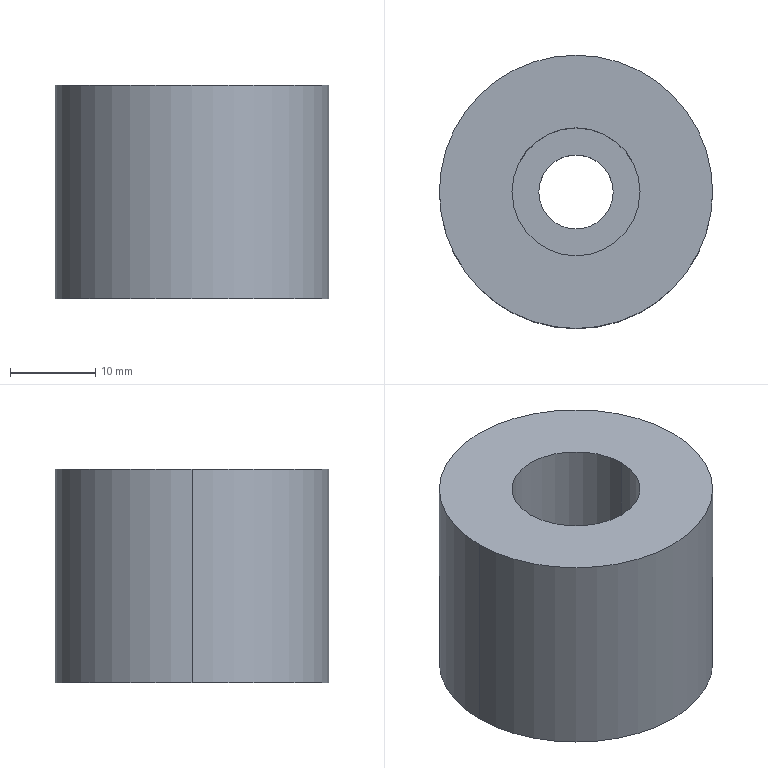Part | STEP file | 1_id1246_x_t | 1 solid | 9 faces | box 32 x 32 x 25 mm | volume 17096 mm3 | cylinder 6 | plane 3 | commonest cylinder face diameters 8.7 x2 15 x2 32 x2
STEP:
#1=CARTESIAN_POINT('',(0.,0.,0.));
#2=DIRECTION('',(0.,0.,1.));
#3=DIRECTION('',(1.,0.,0.));
#4=AXIS2_PLACEMENT_3D('',#1,#2,#3);
#5=CARTESIAN_POINT('',(181.925,338.,3.24));
#6=VERTEX_POINT('',#5);
#7=CARTESIAN_POINT('',(181.925,338.,-21.76));
#8=VERTEX_POINT('',#7);
#9=CARTESIAN_POINT('',(181.925,338.,3.24));
#10=DIRECTION('',(0.,0.,-1.));
#11=VECTOR('',#10,1.);
#12=LINE('',#9,#11);
#13=CARTESIAN_POINT('',(197.925,338.,-46.76));
#14=DIRECTION('',(0.,0.,-1.));
#15=DIRECTION('',(1.,0.,0.));
#16=AXIS2_PLACEMENT_3D('',#13,#14,#15);
#17=CYLINDRICAL_SURFACE('',#16,16.);
#18=CARTESIAN_POINT('',(3.142,-50.));
#19=DIRECTION('',(0.,1.));
#20=VECTOR('',#19,1.);
#21=LINE('',#18,#20);
#22=(GEOMETRIC_REPRESENTATION_CONTEXT(2)PARAMETRIC_REPRESENTATION_CONTEXT()REPRESENTATION_CONTEXT('',''));
#23=DEFINITIONAL_REPRESENTATION('',(#21),#22);
#24=PCURVE('',#17,#23);
#25=CARTESIAN_POINT('',(197.925,338.,-46.76));
#26=DIRECTION('',(0.,0.,-1.));
#27=DIRECTION('',(1.,0.,0.));
#28=AXIS2_PLACEMENT_3D('',#25,#26,#27);
#29=CYLINDRICAL_SURFACE('',#28,16.);
#30=CARTESIAN_POINT('',(3.142,-50.));
#31=DIRECTION('',(0.,1.));
#32=VECTOR('',#31,1.);
#33=LINE('',#30,#32);
#34=(GEOMETRIC_REPRESENTATION_CONTEXT(2)PARAMETRIC_REPRESENTATION_CONTEXT()REPRESENTATION_CONTEXT('',''));
#35=DEFINITIONAL_REPRESENTATION('',(#33),#34);
#36=PCURVE('',#29,#35);
#37=SURFACE_CURVE('',#12,(#24,#36),.PCURVE_S1.);
#38=EDGE_CURVE('',#6,#8,#37,.T.);
#39=ORIENTED_EDGE('',*,*,#38,.F.);
#40=CARTESIAN_POINT('',(213.925,338.,3.24));
#41=VERTEX_POINT('',#40);
#42=CARTESIAN_POINT('',(197.925,338.,3.24));
#43=DIRECTION('',(0.,0.,1.));
#44=DIRECTION('',(1.,0.,0.));
#45=AXIS2_PLACEMENT_3D('',#42,#43,#44);
#46=CIRCLE('',#45,16.);
#47=CARTESIAN_POINT('',(6.283,-50.));
#48=DIRECTION('',(-1.,0.));
#49=VECTOR('',#48,1.);
#50=LINE('',#47,#49);
#51=(GEOMETRIC_REPRESENTATION_CONTEXT(2)PARAMETRIC_REPRESENTATION_CONTEXT()REPRESENTATION_CONTEXT('',''));
#52=DEFINITIONAL_REPRESENTATION('',(#50),#51);
#53=PCURVE('',#17,#52);
#54=CARTESIAN_POINT('',(197.925,338.,3.24));
#55=DIRECTION('',(0.,0.,-1.));
#56=DIRECTION('',(-1.,0.,0.));
#57=AXIS2_PLACEMENT_3D('',#54,#55,#56);
#58=PLANE('',#57);
#59=CARTESIAN_POINT('',(-16.,0.));
#60=CARTESIAN_POINT('',(-16.,27.713));
#61=CARTESIAN_POINT('',(8.,13.856));
#62=CARTESIAN_POINT('',(32.,0.));
#63=CARTESIAN_POINT('',(8.,-13.856));
#64=CARTESIAN_POINT('',(-16.,-27.713));
#65=CARTESIAN_POINT('',(-16.,0.));
#66=(BOUNDED_CURVE()B_SPLINE_CURVE(2,(#59,#60,#61,#62,#63,#64,#65),.UNSPECIFIED.,.T.,.F.)B_SPLINE_CURVE_WITH_KNOTS((1,2,2,2,2,1),(-2.094,0.,2.094,4.189,6.283,8.378),.UNSPECIFIED.)CURVE()GEOMETRIC_REPRESENTATION_ITEM()RATIONAL_B_SPLINE_CURVE((1.,0.5,1.,0.5,1.,0.5,1.))REPRESENTATION_ITEM(''));
#67=(GEOMETRIC_REPRESENTATION_CONTEXT(2)PARAMETRIC_REPRESENTATION_CONTEXT()REPRESENTATION_CONTEXT('',''));
#68=DEFINITIONAL_REPRESENTATION('',(#66),#67);
#69=PCURVE('',#58,#68);
#70=SURFACE_CURVE('',#46,(#53,#69),.PCURVE_S1.);
#71=EDGE_CURVE('',#41,#6,#70,.T.);
#72=ORIENTED_EDGE('',*,*,#71,.F.);
#73=CARTESIAN_POINT('',(213.925,338.,-21.76));
#74=VERTEX_POINT('',#73);
#75=CARTESIAN_POINT('',(213.925,338.,3.24));
#76=DIRECTION('',(0.,0.,1.));
#77=VECTOR('',#76,1.);
#78=LINE('',#75,#77);
#79=CARTESIAN_POINT('',(6.283,-50.));
#80=DIRECTION('',(0.,-1.));
#81=VECTOR('',#80,1.);
#82=LINE('',#79,#81);
#83=(GEOMETRIC_REPRESENTATION_CONTEXT(2)PARAMETRIC_REPRESENTATION_CONTEXT()REPRESENTATION_CONTEXT('',''));
#84=DEFINITIONAL_REPRESENTATION('',(#82),#83);
#85=PCURVE('',#17,#84);
#86=CARTESIAN_POINT('',(0.,-50.));
#87=DIRECTION('',(0.,-1.));
#88=VECTOR('',#87,1.);
#89=LINE('',#86,#88);
#90=(GEOMETRIC_REPRESENTATION_CONTEXT(2)PARAMETRIC_REPRESENTATION_CONTEXT()REPRESENTATION_CONTEXT('',''));
#91=DEFINITIONAL_REPRESENTATION('',(#89),#90);
#92=PCURVE('',#29,#91);
#93=SURFACE_CURVE('',#78,(#85,#92),.PCURVE_S1.);
#94=EDGE_CURVE('',#74,#41,#93,.T.);
#95=ORIENTED_EDGE('',*,*,#94,.F.);
#96=CARTESIAN_POINT('',(197.925,338.,-21.76));
#97=DIRECTION('',(0.,0.,-1.));
#98=DIRECTION('',(-1.,0.,0.));
#99=AXIS2_PLACEMENT_3D('',#96,#97,#98);
#100=CIRCLE('',#99,16.);
#101=CARTESIAN_POINT('',(3.142,-25.));
#102=DIRECTION('',(1.,0.));
#103=VECTOR('',#102,1.);
#104=LINE('',#101,#103);
#105=(GEOMETRIC_REPRESENTATION_CONTEXT(2)PARAMETRIC_REPRESENTATION_CONTEXT()REPRESENTATION_CONTEXT('',''));
#106=DEFINITIONAL_REPRESENTATION('',(#104),#105);
#107=PCURVE('',#17,#106);
#108=CARTESIAN_POINT('',(197.925,338.,-21.76));
#109=DIRECTION('',(0.,0.,1.));
#110=DIRECTION('',(1.,0.,0.));
#111=AXIS2_PLACEMENT_3D('',#108,#109,#110);
#112=PLANE('',#111);
#113=CARTESIAN_POINT('',(-16.,0.));
#114=CARTESIAN_POINT('',(-16.,27.713));
#115=CARTESIAN_POINT('',(8.,13.856));
#116=CARTESIAN_POINT('',(32.,0.));
#117=CARTESIAN_POINT('',(8.,-13.856));
#118=CARTESIAN_POINT('',(-16.,-27.713));
#119=CARTESIAN_POINT('',(-16.,0.));
#120=(BOUNDED_CURVE()B_SPLINE_CURVE(2,(#113,#114,#115,#116,#117,#118,#119),.UNSPECIFIED.,.T.,.F.)B_SPLINE_CURVE_WITH_KNOTS((1,2,2,2,2,1),(-2.094,0.,2.094,4.189,6.283,8.378),.UNSPECIFIED.)CURVE()GEOMETRIC_REPRESENTATION_ITEM()RATIONAL_B_SPLINE_CURVE((1.,0.5,1.,0.5,1.,0.5,1.))REPRESENTATION_ITEM(''));
#121=(GEOMETRIC_REPRESENTATION_CONTEXT(2)PARAMETRIC_REPRESENTATION_CONTEXT()REPRESENTATION_CONTEXT('',''));
#122=DEFINITIONAL_REPRESENTATION('',(#120),#121);
#123=PCURVE('',#112,#122);
#124=SURFACE_CURVE('',#100,(#107,#123),.PCURVE_S1.);
#125=EDGE_CURVE('',#8,#74,#124,.T.);
#126=ORIENTED_EDGE('',*,*,#125,.F.);
#127=EDGE_LOOP('',(#39,#72,#95,#126));
#128=FACE_BOUND('',#127,.T.);
#129=ADVANCED_FACE('',(#128),#17,.T.);
#130=CARTESIAN_POINT('',(197.925,338.,-21.76));
#131=DIRECTION('',(0.,0.,-1.));
#132=DIRECTION('',(1.,0.,0.));
#133=AXIS2_PLACEMENT_3D('',#130,#131,#132);
#134=CIRCLE('',#133,16.);
#135=CARTESIAN_POINT('',(16.,0.));
#136=CARTESIAN_POINT('',(16.,-27.713));
#137=CARTESIAN_POINT('',(-8.,-13.856));
#138=CARTESIAN_POINT('',(-32.,0.));
#139=CARTESIAN_POINT('',(-8.,13.856));
#140=CARTESIAN_POINT('',(16.,27.713));
#141=CARTESIAN_POINT('',(16.,0.));
#142=(BOUNDED_CURVE()B_SPLINE_CURVE(2,(#135,#136,#137,#138,#139,#140,#141),.UNSPECIFIED.,.T.,.F.)B_SPLINE_CURVE_WITH_KNOTS((1,2,2,2,2,1),(-2.094,0.,2.094,4.189,6.283,8.378),.UNSPECIFIED.)CURVE()GEOMETRIC_REPRESENTATION_ITEM()RATIONAL_B_SPLINE_CURVE((1.,0.5,1.,0.5,1.,0.5,1.))REPRESENTATION_ITEM(''));
#143=(GEOMETRIC_REPRESENTATION_CONTEXT(2)PARAMETRIC_REPRESENTATION_CONTEXT()REPRESENTATION_CONTEXT('',''));
#144=DEFINITIONAL_REPRESENTATION('',(#142),#143);
#145=PCURVE('',#112,#144);
#146=CARTESIAN_POINT('',(0.,-25.));
#147=DIRECTION('',(1.,0.));
#148=VECTOR('',#147,1.);
#149=LINE('',#146,#148);
#150=(GEOMETRIC_REPRESENTATION_CONTEXT(2)PARAMETRIC_REPRESENTATION_CONTEXT()REPRESENTATION_CONTEXT('',''));
#151=DEFINITIONAL_REPRESENTATION('',(#149),#150);
#152=PCURVE('',#29,#151);
#153=SURFACE_CURVE('',#134,(#145,#152),.PCURVE_S1.);
#154=EDGE_CURVE('',#74,#8,#153,.T.);
#155=ORIENTED_EDGE('',*,*,#154,.T.);
#156=ORIENTED_EDGE('',*,*,#125,.T.);
#157=EDGE_LOOP('',(#155,#156));
#158=FACE_BOUND('',#157,.T.);
#159=CARTESIAN_POINT('',(202.275,338.,-21.76));
#160=VERTEX_POINT('',#159);
#161=CARTESIAN_POINT('',(193.575,338.,-21.76));
#162=VERTEX_POINT('',#161);
#163=CARTESIAN_POINT('',(197.925,338.,-21.76));
#164=DIRECTION('',(0.,0.,1.));
#165=DIRECTION('',(1.,0.,0.));
#166=AXIS2_PLACEMENT_3D('',#163,#164,#165);
#167=CIRCLE('',#166,4.35);
#168=CARTESIAN_POINT('',(0.,0.));
#169=DIRECTION('',(1.,0.));
#170=AXIS2_PLACEMENT_2D('',#168,#169);
#171=CIRCLE('',#170,4.35);
#172=(GEOMETRIC_REPRESENTATION_CONTEXT(2)PARAMETRIC_REPRESENTATION_CONTEXT()REPRESENTATION_CONTEXT('',''));
#173=DEFINITIONAL_REPRESENTATION('',(#171),#172);
#174=PCURVE('',#112,#173);
#175=CARTESIAN_POINT('',(197.925,338.,-47.26));
#176=DIRECTION('',(0.,0.,-1.));
#177=DIRECTION('',(1.,0.,0.));
#178=AXIS2_PLACEMENT_3D('',#175,#176,#177);
#179=CYLINDRICAL_SURFACE('',#178,4.35);
#180=CARTESIAN_POINT('',(6.283,-25.5));
#181=DIRECTION('',(-1.,0.));
#182=VECTOR('',#181,1.);
#183=LINE('',#180,#182);
#184=(GEOMETRIC_REPRESENTATION_CONTEXT(2)PARAMETRIC_REPRESENTATION_CONTEXT()REPRESENTATION_CONTEXT('',''));
#185=DEFINITIONAL_REPRESENTATION('',(#183),#184);
#186=PCURVE('',#179,#185);
#187=SURFACE_CURVE('',#167,(#174,#186),.PCURVE_S1.);
#188=EDGE_CURVE('',#160,#162,#187,.T.);
#189=ORIENTED_EDGE('',*,*,#188,.T.);
#190=CARTESIAN_POINT('',(197.925,338.,-21.76));
#191=DIRECTION('',(0.,0.,1.));
#192=DIRECTION('',(-1.,0.,0.));
#193=AXIS2_PLACEMENT_3D('',#190,#191,#192);
#194=CIRCLE('',#193,4.35);
#195=CARTESIAN_POINT('',(0.,0.));
#196=DIRECTION('',(-1.,0.));
#197=AXIS2_PLACEMENT_2D('',#195,#196);
#198=CIRCLE('',#197,4.35);
#199=(GEOMETRIC_REPRESENTATION_CONTEXT(2)PARAMETRIC_REPRESENTATION_CONTEXT()REPRESENTATION_CONTEXT('',''));
#200=DEFINITIONAL_REPRESENTATION('',(#198),#199);
#201=PCURVE('',#112,#200);
#202=CARTESIAN_POINT('',(197.925,338.,-47.26));
#203=DIRECTION('',(0.,0.,-1.));
#204=DIRECTION('',(1.,0.,0.));
#205=AXIS2_PLACEMENT_3D('',#202,#203,#204);
#206=CYLINDRICAL_SURFACE('',#205,4.35);
#207=CARTESIAN_POINT('',(3.142,-25.5));
#208=DIRECTION('',(-1.,0.));
#209=VECTOR('',#208,1.);
#210=LINE('',#207,#209);
#211=(GEOMETRIC_REPRESENTATION_CONTEXT(2)PARAMETRIC_REPRESENTATION_CONTEXT()REPRESENTATION_CONTEXT('',''));
#212=DEFINITIONAL_REPRESENTATION('',(#210),#211);
#213=PCURVE('',#206,#212);
#214=SURFACE_CURVE('',#194,(#201,#213),.PCURVE_S1.);
#215=EDGE_CURVE('',#162,#160,#214,.T.);
#216=ORIENTED_EDGE('',*,*,#215,.T.);
#217=EDGE_LOOP('',(#189,#216));
#218=FACE_BOUND('',#217,.T.);
#219=ADVANCED_FACE('',(#158,#218),#112,.F.);
#220=ORIENTED_EDGE('',*,*,#94,.T.);
#221=CARTESIAN_POINT('',(197.925,338.,3.24));
#222=DIRECTION('',(0.,0.,1.));
#223=DIRECTION('',(-1.,0.,0.));
#224=AXIS2_PLACEMENT_3D('',#221,#222,#223);
#225=CIRCLE('',#224,16.);
#226=CARTESIAN_POINT('',(3.142,-50.));
#227=DIRECTION('',(-1.,0.));
#228=VECTOR('',#227,1.);
#229=LINE('',#226,#228);
#230=(GEOMETRIC_REPRESENTATION_CONTEXT(2)PARAMETRIC_REPRESENTATION_CONTEXT()REPRESENTATION_CONTEXT('',''));
#231=DEFINITIONAL_REPRESENTATION('',(#229),#230);
#232=PCURVE('',#29,#231);
#233=CARTESIAN_POINT('',(16.,0.));
#234=CARTESIAN_POINT('',(16.,-27.713));
#235=CARTESIAN_POINT('',(-8.,-13.856));
#236=CARTESIAN_POINT('',(-32.,0.));
#237=CARTESIAN_POINT('',(-8.,13.856));
#238=CARTESIAN_POINT('',(16.,27.713));
#239=CARTESIAN_POINT('',(16.,0.));
#240=(BOUNDED_CURVE()B_SPLINE_CURVE(2,(#233,#234,#235,#236,#237,#238,#239),.UNSPECIFIED.,.T.,.F.)B_SPLINE_CURVE_WITH_KNOTS((1,2,2,2,2,1),(-2.094,0.,2.094,4.189,6.283,8.378),.UNSPECIFIED.)CURVE()GEOMETRIC_REPRESENTATION_ITEM()RATIONAL_B_SPLINE_CURVE((1.,0.5,1.,0.5,1.,0.5,1.))REPRESENTATION_ITEM(''));
#241=(GEOMETRIC_REPRESENTATION_CONTEXT(2)PARAMETRIC_REPRESENTATION_CONTEXT()REPRESENTATION_CONTEXT('',''));
#242=DEFINITIONAL_REPRESENTATION('',(#240),#241);
#243=PCURVE('',#58,#242);
#244=SURFACE_CURVE('',#225,(#232,#243),.PCURVE_S1.);
#245=EDGE_CURVE('',#6,#41,#244,.T.);
#246=ORIENTED_EDGE('',*,*,#245,.F.);
#247=ORIENTED_EDGE('',*,*,#38,.T.);
#248=ORIENTED_EDGE('',*,*,#154,.F.);
#249=EDGE_LOOP('',(#220,#246,#247,#248));
#250=FACE_BOUND('',#249,.T.);
#251=ADVANCED_FACE('',(#250),#29,.T.);
#252=ORIENTED_EDGE('',*,*,#71,.T.);
#253=ORIENTED_EDGE('',*,*,#245,.T.);
#254=EDGE_LOOP('',(#252,#253));
#255=FACE_BOUND('',#254,.T.);
#256=CARTESIAN_POINT('',(205.425,338.,3.24));
#257=VERTEX_POINT('',#256);
#258=CARTESIAN_POINT('',(190.425,338.,3.24));
#259=VERTEX_POINT('',#258);
#260=CARTESIAN_POINT('',(197.925,338.,3.24));
#261=DIRECTION('',(0.,0.,-1.));
#262=DIRECTION('',(1.,0.,0.));
#263=AXIS2_PLACEMENT_3D('',#260,#261,#262);
#264=CIRCLE('',#263,7.5);
#265=CARTESIAN_POINT('',(0.,0.));
#266=DIRECTION('',(-1.,0.));
#267=AXIS2_PLACEMENT_2D('',#265,#266);
#268=CIRCLE('',#267,7.5);
#269=(GEOMETRIC_REPRESENTATION_CONTEXT(2)PARAMETRIC_REPRESENTATION_CONTEXT()REPRESENTATION_CONTEXT('',''));
#270=DEFINITIONAL_REPRESENTATION('',(#268),#269);
#271=PCURVE('',#58,#270);
#272=CARTESIAN_POINT('',(197.925,338.,-9.76));
#273=DIRECTION('',(0.,0.,-1.));
#274=DIRECTION('',(1.,0.,0.));
#275=AXIS2_PLACEMENT_3D('',#272,#273,#274);
#276=CYLINDRICAL_SURFACE('',#275,7.5);
#277=CARTESIAN_POINT('',(0.,-13.));
#278=DIRECTION('',(1.,0.));
#279=VECTOR('',#278,1.);
#280=LINE('',#277,#279);
#281=(GEOMETRIC_REPRESENTATION_CONTEXT(2)PARAMETRIC_REPRESENTATION_CONTEXT()REPRESENTATION_CONTEXT('',''));
#282=DEFINITIONAL_REPRESENTATION('',(#280),#281);
#283=PCURVE('',#276,#282);
#284=SURFACE_CURVE('',#264,(#271,#283),.PCURVE_S1.);
#285=EDGE_CURVE('',#257,#259,#284,.T.);
#286=ORIENTED_EDGE('',*,*,#285,.T.);
#287=CARTESIAN_POINT('',(197.925,338.,3.24));
#288=DIRECTION('',(0.,0.,-1.));
#289=DIRECTION('',(-1.,0.,0.));
#290=AXIS2_PLACEMENT_3D('',#287,#288,#289);
#291=CIRCLE('',#290,7.5);
#292=CARTESIAN_POINT('',(0.,0.));
#293=DIRECTION('',(1.,0.));
#294=AXIS2_PLACEMENT_2D('',#292,#293);
#295=CIRCLE('',#294,7.5);
#296=(GEOMETRIC_REPRESENTATION_CONTEXT(2)PARAMETRIC_REPRESENTATION_CONTEXT()REPRESENTATION_CONTEXT('',''));
#297=DEFINITIONAL_REPRESENTATION('',(#295),#296);
#298=PCURVE('',#58,#297);
#299=CARTESIAN_POINT('',(197.925,338.,-9.76));
#300=DIRECTION('',(0.,0.,-1.));
#301=DIRECTION('',(1.,0.,0.));
#302=AXIS2_PLACEMENT_3D('',#299,#300,#301);
#303=CYLINDRICAL_SURFACE('',#302,7.5);
#304=CARTESIAN_POINT('',(3.142,-13.));
#305=DIRECTION('',(1.,0.));
#306=VECTOR('',#305,1.);
#307=LINE('',#304,#306);
#308=(GEOMETRIC_REPRESENTATION_CONTEXT(2)PARAMETRIC_REPRESENTATION_CONTEXT()REPRESENTATION_CONTEXT('',''));
#309=DEFINITIONAL_REPRESENTATION('',(#307),#308);
#310=PCURVE('',#303,#309);
#311=SURFACE_CURVE('',#291,(#298,#310),.PCURVE_S1.);
#312=EDGE_CURVE('',#259,#257,#311,.T.);
#313=ORIENTED_EDGE('',*,*,#312,.T.);
#314=EDGE_LOOP('',(#286,#313));
#315=FACE_BOUND('',#314,.T.);
#316=ADVANCED_FACE('',(#255,#315),#58,.F.);
#317=CARTESIAN_POINT('',(205.425,338.,-9.76));
#318=VERTEX_POINT('',#317);
#319=CARTESIAN_POINT('',(190.425,338.,-9.76));
#320=VERTEX_POINT('',#319);
#321=CARTESIAN_POINT('',(197.925,338.,-9.76));
#322=DIRECTION('',(0.,0.,1.));
#323=DIRECTION('',(1.,0.,0.));
#324=AXIS2_PLACEMENT_3D('',#321,#322,#323);
#325=CIRCLE('',#324,7.5);
#326=CARTESIAN_POINT('',(6.283,0.));
#327=DIRECTION('',(-1.,0.));
#328=VECTOR('',#327,1.);
#329=LINE('',#326,#328);
#330=(GEOMETRIC_REPRESENTATION_CONTEXT(2)PARAMETRIC_REPRESENTATION_CONTEXT()REPRESENTATION_CONTEXT('',''));
#331=DEFINITIONAL_REPRESENTATION('',(#329),#330);
#332=PCURVE('',#303,#331);
#333=CARTESIAN_POINT('',(197.925,338.,-9.76));
#334=DIRECTION('',(0.,0.,-1.));
#335=DIRECTION('',(-1.,0.,0.));
#336=AXIS2_PLACEMENT_3D('',#333,#334,#335);
#337=PLANE('',#336);
#338=CARTESIAN_POINT('',(-7.5,0.));
#339=CARTESIAN_POINT('',(-7.5,12.99));
#340=CARTESIAN_POINT('',(3.75,6.495));
#341=CARTESIAN_POINT('',(15.,0.));
#342=CARTESIAN_POINT('',(3.75,-6.495));
#343=CARTESIAN_POINT('',(-7.5,-12.99));
#344=CARTESIAN_POINT('',(-7.5,0.));
#345=(BOUNDED_CURVE()B_SPLINE_CURVE(2,(#338,#339,#340,#341,#342,#343,#344),.UNSPECIFIED.,.T.,.F.)B_SPLINE_CURVE_WITH_KNOTS((1,2,2,2,2,1),(-2.094,0.,2.094,4.189,6.283,8.378),.UNSPECIFIED.)CURVE()GEOMETRIC_REPRESENTATION_ITEM()RATIONAL_B_SPLINE_CURVE((1.,0.5,1.,0.5,1.,0.5,1.))REPRESENTATION_ITEM(''));
#346=(GEOMETRIC_REPRESENTATION_CONTEXT(2)PARAMETRIC_REPRESENTATION_CONTEXT()REPRESENTATION_CONTEXT('',''));
#347=DEFINITIONAL_REPRESENTATION('',(#345),#346);
#348=PCURVE('',#337,#347);
#349=SURFACE_CURVE('',#325,(#332,#348),.PCURVE_S1.);
#350=EDGE_CURVE('',#318,#320,#349,.T.);
#351=ORIENTED_EDGE('',*,*,#350,.T.);
#352=CARTESIAN_POINT('',(190.425,338.,3.24));
#353=DIRECTION('',(0.,0.,-1.));
#354=VECTOR('',#353,1.);
#355=LINE('',#352,#354);
#356=CARTESIAN_POINT('',(3.142,-13.));
#357=DIRECTION('',(0.,1.));
#358=VECTOR('',#357,1.);
#359=LINE('',#356,#358);
#360=(GEOMETRIC_REPRESENTATION_CONTEXT(2)PARAMETRIC_REPRESENTATION_CONTEXT()REPRESENTATION_CONTEXT('',''));
#361=DEFINITIONAL_REPRESENTATION('',(#359),#360);
#362=PCURVE('',#303,#361);
#363=CARTESIAN_POINT('',(3.142,-13.));
#364=DIRECTION('',(0.,1.));
#365=VECTOR('',#364,1.);
#366=LINE('',#363,#365);
#367=(GEOMETRIC_REPRESENTATION_CONTEXT(2)PARAMETRIC_REPRESENTATION_CONTEXT()REPRESENTATION_CONTEXT('',''));
#368=DEFINITIONAL_REPRESENTATION('',(#366),#367);
#369=PCURVE('',#276,#368);
#370=SURFACE_CURVE('',#355,(#362,#369),.PCURVE_S1.);
#371=EDGE_CURVE('',#259,#320,#370,.T.);
#372=ORIENTED_EDGE('',*,*,#371,.F.);
#373=ORIENTED_EDGE('',*,*,#312,.T.);
#374=CARTESIAN_POINT('',(205.425,338.,3.24));
#375=DIRECTION('',(0.,0.,1.));
#376=VECTOR('',#375,1.);
#377=LINE('',#374,#376);
#378=CARTESIAN_POINT('',(6.283,-13.));
#379=DIRECTION('',(0.,-1.));
#380=VECTOR('',#379,1.);
#381=LINE('',#378,#380);
#382=(GEOMETRIC_REPRESENTATION_CONTEXT(2)PARAMETRIC_REPRESENTATION_CONTEXT()REPRESENTATION_CONTEXT('',''));
#383=DEFINITIONAL_REPRESENTATION('',(#381),#382);
#384=PCURVE('',#303,#383);
#385=CARTESIAN_POINT('',(0.,-13.));
#386=DIRECTION('',(0.,-1.));
#387=VECTOR('',#386,1.);
#388=LINE('',#385,#387);
#389=(GEOMETRIC_REPRESENTATION_CONTEXT(2)PARAMETRIC_REPRESENTATION_CONTEXT()REPRESENTATION_CONTEXT('',''));
#390=DEFINITIONAL_REPRESENTATION('',(#388),#389);
#391=PCURVE('',#276,#390);
#392=SURFACE_CURVE('',#377,(#384,#391),.PCURVE_S1.);
#393=EDGE_CURVE('',#318,#257,#392,.T.);
#394=ORIENTED_EDGE('',*,*,#393,.F.);
#395=EDGE_LOOP('',(#351,#372,#373,#394));
#396=FACE_BOUND('',#395,.F.);
#397=ADVANCED_FACE('',(#396),#303,.F.);
#398=ORIENTED_EDGE('',*,*,#350,.T.);
#399=CARTESIAN_POINT('',(197.925,338.,-9.76));
#400=DIRECTION('',(0.,0.,1.));
#401=DIRECTION('',(-1.,0.,0.));
#402=AXIS2_PLACEMENT_3D('',#399,#400,#401);
#403=CIRCLE('',#402,7.5);
#404=CARTESIAN_POINT('',(7.5,0.));
#405=CARTESIAN_POINT('',(7.5,-12.99));
#406=CARTESIAN_POINT('',(-3.75,-6.495));
#407=CARTESIAN_POINT('',(-15.,0.));
#408=CARTESIAN_POINT('',(-3.75,6.495));
#409=CARTESIAN_POINT('',(7.5,12.99));
#410=CARTESIAN_POINT('',(7.5,0.));
#411=(BOUNDED_CURVE()B_SPLINE_CURVE(2,(#404,#405,#406,#407,#408,#409,#410),.UNSPECIFIED.,.T.,.F.)B_SPLINE_CURVE_WITH_KNOTS((1,2,2,2,2,1),(-2.094,0.,2.094,4.189,6.283,8.378),.UNSPECIFIED.)CURVE()GEOMETRIC_REPRESENTATION_ITEM()RATIONAL_B_SPLINE_CURVE((1.,0.5,1.,0.5,1.,0.5,1.))REPRESENTATION_ITEM(''));
#412=(GEOMETRIC_REPRESENTATION_CONTEXT(2)PARAMETRIC_REPRESENTATION_CONTEXT()REPRESENTATION_CONTEXT('',''));
#413=DEFINITIONAL_REPRESENTATION('',(#411),#412);
#414=PCURVE('',#337,#413);
#415=CARTESIAN_POINT('',(3.142,0.));
#416=DIRECTION('',(-1.,0.));
#417=VECTOR('',#416,1.);
#418=LINE('',#415,#417);
#419=(GEOMETRIC_REPRESENTATION_CONTEXT(2)PARAMETRIC_REPRESENTATION_CONTEXT()REPRESENTATION_CONTEXT('',''));
#420=DEFINITIONAL_REPRESENTATION('',(#418),#419);
#421=PCURVE('',#276,#420);
#422=SURFACE_CURVE('',#403,(#414,#421),.PCURVE_S1.);
#423=EDGE_CURVE('',#320,#318,#422,.T.);
#424=ORIENTED_EDGE('',*,*,#423,.T.);
#425=EDGE_LOOP('',(#398,#424));
#426=FACE_BOUND('',#425,.T.);
#427=CARTESIAN_POINT('',(193.575,338.,-9.76));
#428=VERTEX_POINT('',#427);
#429=CARTESIAN_POINT('',(202.275,338.,-9.76));
#430=VERTEX_POINT('',#429);
#431=CARTESIAN_POINT('',(197.925,338.,-9.76));
#432=DIRECTION('',(0.,0.,-1.));
#433=DIRECTION('',(-1.,0.,0.));
#434=AXIS2_PLACEMENT_3D('',#431,#432,#433);
#435=CIRCLE('',#434,4.35);
#436=CARTESIAN_POINT('',(0.,0.));
#437=DIRECTION('',(1.,0.));
#438=AXIS2_PLACEMENT_2D('',#436,#437);
#439=CIRCLE('',#438,4.35);
#440=(GEOMETRIC_REPRESENTATION_CONTEXT(2)PARAMETRIC_REPRESENTATION_CONTEXT()REPRESENTATION_CONTEXT('',''));
#441=DEFINITIONAL_REPRESENTATION('',(#439),#440);
#442=PCURVE('',#337,#441);
#443=CARTESIAN_POINT('',(3.142,-37.5));
#444=DIRECTION('',(1.,0.));
#445=VECTOR('',#444,1.);
#446=LINE('',#443,#445);
#447=(GEOMETRIC_REPRESENTATION_CONTEXT(2)PARAMETRIC_REPRESENTATION_CONTEXT()REPRESENTATION_CONTEXT('',''));
#448=DEFINITIONAL_REPRESENTATION('',(#446),#447);
#449=PCURVE('',#179,#448);
#450=SURFACE_CURVE('',#435,(#442,#449),.PCURVE_S1.);
#451=EDGE_CURVE('',#428,#430,#450,.T.);
#452=ORIENTED_EDGE('',*,*,#451,.T.);
#453=CARTESIAN_POINT('',(197.925,338.,-9.76));
#454=DIRECTION('',(0.,0.,-1.));
#455=DIRECTION('',(1.,0.,0.));
#456=AXIS2_PLACEMENT_3D('',#453,#454,#455);
#457=CIRCLE('',#456,4.35);
#458=CARTESIAN_POINT('',(0.,0.));
#459=DIRECTION('',(-1.,0.));
#460=AXIS2_PLACEMENT_2D('',#458,#459);
#461=CIRCLE('',#460,4.35);
#462=(GEOMETRIC_REPRESENTATION_CONTEXT(2)PARAMETRIC_REPRESENTATION_CONTEXT()REPRESENTATION_CONTEXT('',''));
#463=DEFINITIONAL_REPRESENTATION('',(#461),#462);
#464=PCURVE('',#337,#463);
#465=CARTESIAN_POINT('',(0.,-37.5));
#466=DIRECTION('',(1.,0.));
#467=VECTOR('',#466,1.);
#468=LINE('',#465,#467);
#469=(GEOMETRIC_REPRESENTATION_CONTEXT(2)PARAMETRIC_REPRESENTATION_CONTEXT()REPRESENTATION_CONTEXT('',''));
#470=DEFINITIONAL_REPRESENTATION('',(#468),#469);
#471=PCURVE('',#206,#470);
#472=SURFACE_CURVE('',#457,(#464,#471),.PCURVE_S1.);
#473=EDGE_CURVE('',#430,#428,#472,.T.);
#474=ORIENTED_EDGE('',*,*,#473,.T.);
#475=EDGE_LOOP('',(#452,#474));
#476=FACE_BOUND('',#475,.T.);
#477=ADVANCED_FACE('',(#426,#476),#337,.F.);
#478=ORIENTED_EDGE('',*,*,#423,.T.);
#479=ORIENTED_EDGE('',*,*,#393,.T.);
#480=ORIENTED_EDGE('',*,*,#285,.T.);
#481=ORIENTED_EDGE('',*,*,#371,.T.);
#482=EDGE_LOOP('',(#478,#479,#480,#481));
#483=FACE_BOUND('',#482,.F.);
#484=ADVANCED_FACE('',(#483),#276,.F.);
#485=ORIENTED_EDGE('',*,*,#215,.T.);
#486=CARTESIAN_POINT('',(202.275,338.,-9.76));
#487=DIRECTION('',(0.,0.,-1.));
#488=VECTOR('',#487,1.);
#489=LINE('',#486,#488);
#490=CARTESIAN_POINT('',(0.,-37.5));
#491=DIRECTION('',(0.,1.));
#492=VECTOR('',#491,1.);
#493=LINE('',#490,#492);
#494=(GEOMETRIC_REPRESENTATION_CONTEXT(2)PARAMETRIC_REPRESENTATION_CONTEXT()REPRESENTATION_CONTEXT('',''));
#495=DEFINITIONAL_REPRESENTATION('',(#493),#494);
#496=PCURVE('',#206,#495);
#497=CARTESIAN_POINT('',(6.283,-37.5));
#498=DIRECTION('',(0.,1.));
#499=VECTOR('',#498,1.);
#500=LINE('',#497,#499);
#501=(GEOMETRIC_REPRESENTATION_CONTEXT(2)PARAMETRIC_REPRESENTATION_CONTEXT()REPRESENTATION_CONTEXT('',''));
#502=DEFINITIONAL_REPRESENTATION('',(#500),#501);
#503=PCURVE('',#179,#502);
#504=SURFACE_CURVE('',#489,(#496,#503),.PCURVE_S1.);
#505=EDGE_CURVE('',#430,#160,#504,.T.);
#506=ORIENTED_EDGE('',*,*,#505,.F.);
#507=ORIENTED_EDGE('',*,*,#473,.T.);
#508=CARTESIAN_POINT('',(193.575,338.,-9.76));
#509=DIRECTION('',(0.,0.,1.));
#510=VECTOR('',#509,1.);
#511=LINE('',#508,#510);
#512=CARTESIAN_POINT('',(3.142,-37.5));
#513=DIRECTION('',(0.,-1.));
#514=VECTOR('',#513,1.);
#515=LINE('',#512,#514);
#516=(GEOMETRIC_REPRESENTATION_CONTEXT(2)PARAMETRIC_REPRESENTATION_CONTEXT()REPRESENTATION_CONTEXT('',''));
#517=DEFINITIONAL_REPRESENTATION('',(#515),#516);
#518=PCURVE('',#206,#517);
#519=CARTESIAN_POINT('',(3.142,-37.5));
#520=DIRECTION('',(0.,-1.));
#521=VECTOR('',#520,1.);
#522=LINE('',#519,#521);
#523=(GEOMETRIC_REPRESENTATION_CONTEXT(2)PARAMETRIC_REPRESENTATION_CONTEXT()REPRESENTATION_CONTEXT('',''));
#524=DEFINITIONAL_REPRESENTATION('',(#522),#523);
#525=PCURVE('',#179,#524);
#526=SURFACE_CURVE('',#511,(#518,#525),.PCURVE_S1.);
#527=EDGE_CURVE('',#162,#428,#526,.T.);
#528=ORIENTED_EDGE('',*,*,#527,.F.);
#529=EDGE_LOOP('',(#485,#506,#507,#528));
#530=FACE_BOUND('',#529,.F.);
#531=ADVANCED_FACE('',(#530),#206,.F.);
#532=ORIENTED_EDGE('',*,*,#188,.T.);
#533=ORIENTED_EDGE('',*,*,#527,.T.);
#534=ORIENTED_EDGE('',*,*,#451,.T.);
#535=ORIENTED_EDGE('',*,*,#505,.T.);
#536=EDGE_LOOP('',(#532,#533,#534,#535));
#537=FACE_BOUND('',#536,.F.);
#538=ADVANCED_FACE('',(#537),#179,.F.);
#539=CLOSED_SHELL('',(#129,#219,#251,#316,#397,#477,#484,#531,#538));
#540=MANIFOLD_SOLID_BREP('',#539);
#541=(LENGTH_UNIT()NAMED_UNIT(*)SI_UNIT(.MILLI.,.METRE.));
#542=UNCERTAINTY_MEASURE_WITH_UNIT(LENGTH_MEASURE(0.0000001),#541,'','');
#543=(NAMED_UNIT(*)PLANE_ANGLE_UNIT()SI_UNIT($,.RADIAN.));
#544=(NAMED_UNIT(*)SI_UNIT($,.STERADIAN.)SOLID_ANGLE_UNIT());
#545=(GEOMETRIC_REPRESENTATION_CONTEXT(3)GLOBAL_UNCERTAINTY_ASSIGNED_CONTEXT((#542))GLOBAL_UNIT_ASSIGNED_CONTEXT((#541,#543,#544))REPRESENTATION_CONTEXT('',''));
#546=ADVANCED_BREP_SHAPE_REPRESENTATION('',(#4,#540),#545);